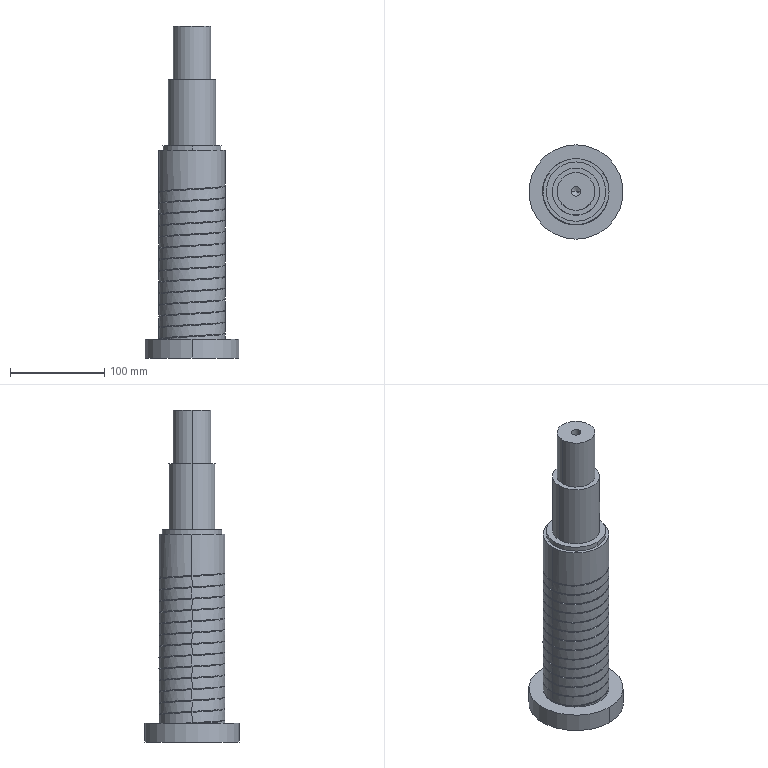Part | SolidWorks | features BaseBody 1 | 1 solid | 50 faces | box 100 x 100 x 352 mm | volume 1147251 mm3 | cylinder 38 | plane 8 | cone 2 | spline 2 | commonest cylinder face diameters 70 x28 10.2 x2 40 x2 50 x2 63 x2 100 x2